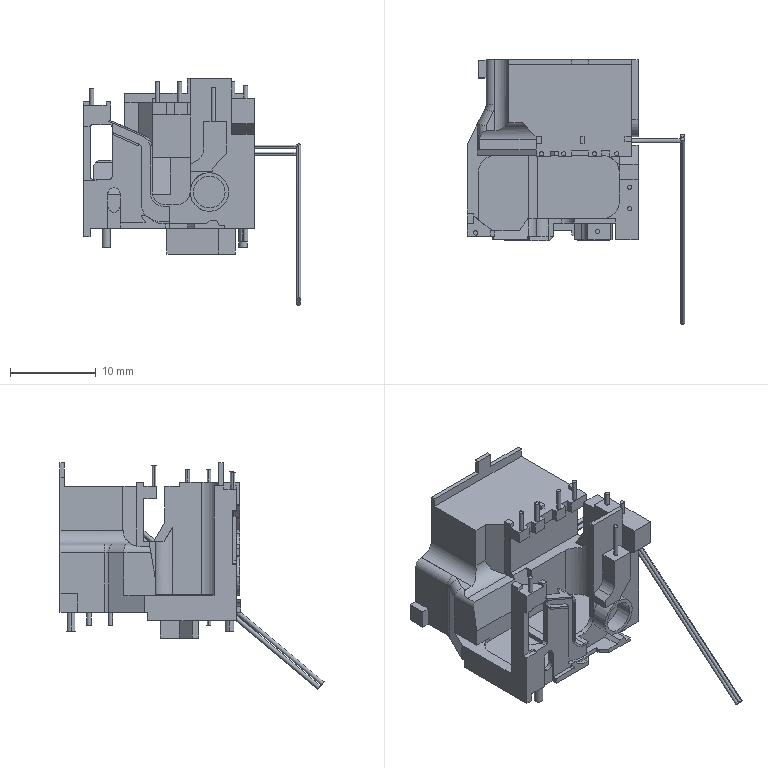Part | NX | features BREP 1 | 1 solid | 525 faces | box 25.45 x 30.878 x 26.482 mm | volume 2338 mm3 | plane 345 | cylinder 92 | spline 87 | torus 1 | commonest cylinder face diameters 0.5 x39 0.1 x10 1 x7 3 x7 4 x5 0.6 x4